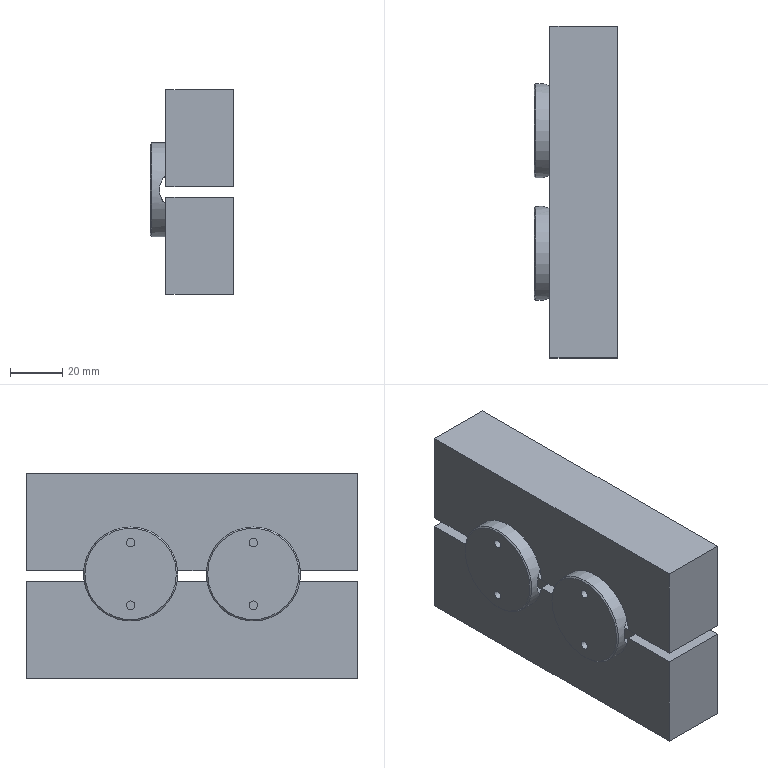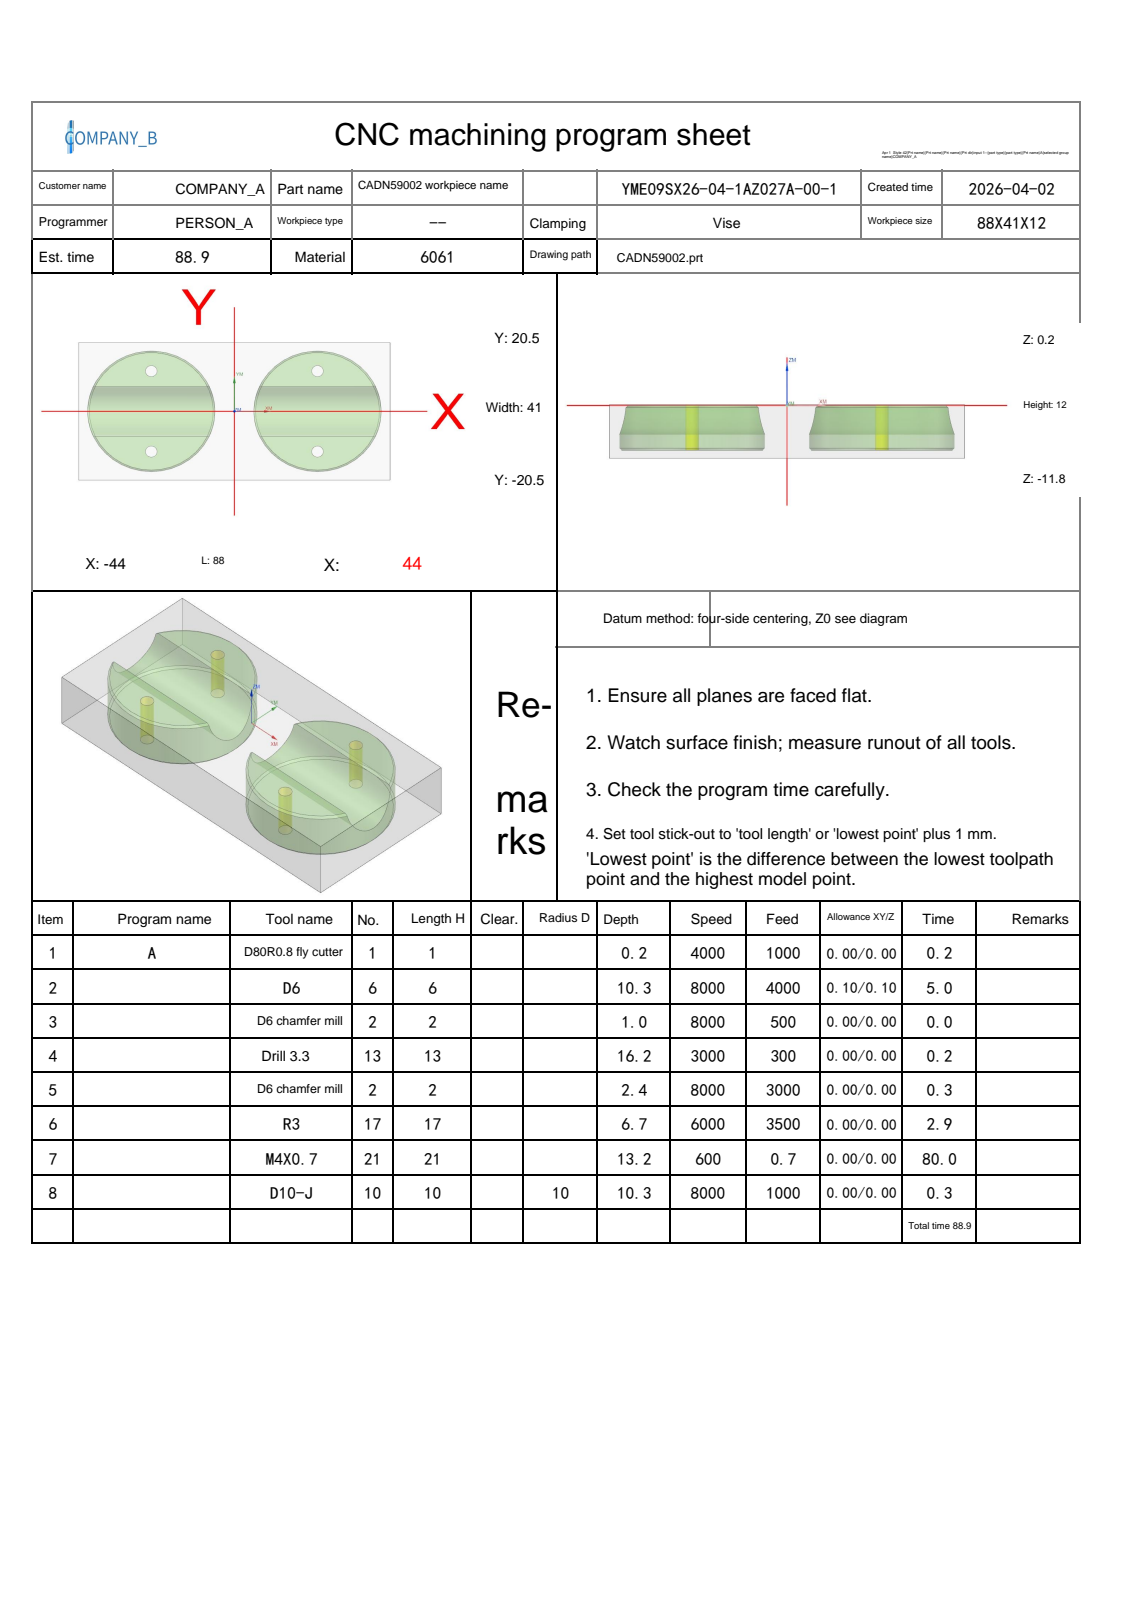NC program | NX | posted by the shop | part box 32 x 127 x 78.432 mm
Lines 1 to 33 of 8369:
%
O0001
(Machine time: 164.82 MIN)
(===Total Tool:7===)
(T1=D80R0.8 fly cutter D=80.  R=0.8  D-  H01 Z=0.    )
(T6=D6      D=6.   R=0.   D-  H06 Z=-10.1 )
(T2=D6 chamfer mill   D=6.   R=0.   D-  H02 Z=-2.2  )
(T13=drill 3.3  D=3.3  DR_a=118 D-  H13 Z=-15.99)
(T17=R3     D=6.   R=3.   D-  H17 Z=-6.5  )
(T21=M4X0.7 D=3.3  DR_a=180 D-  H21 Z=-13.  )
(T10=D10-J  D=10.  R=0.   D10 H10 Z=-10.1 )
G80 G90 G17 G49 G40
G91 G28 Z0
M01
N1 T01 M06
(D80R0.8 fly cutter  D=80. R=0.8 H=01 ce=0.00 di=0.00)
G00 G90 G54 X-86.5 Y0.0 M03 S4000
G43 H01 Z20.
M08
Z2.
G01 Z0.0 F1000.
X-81.5
X81.5
X86.5
Z2.
G00 Z20.
G91 G28 Z0.0
M05
M09
G91 G28 Z0.0
M01